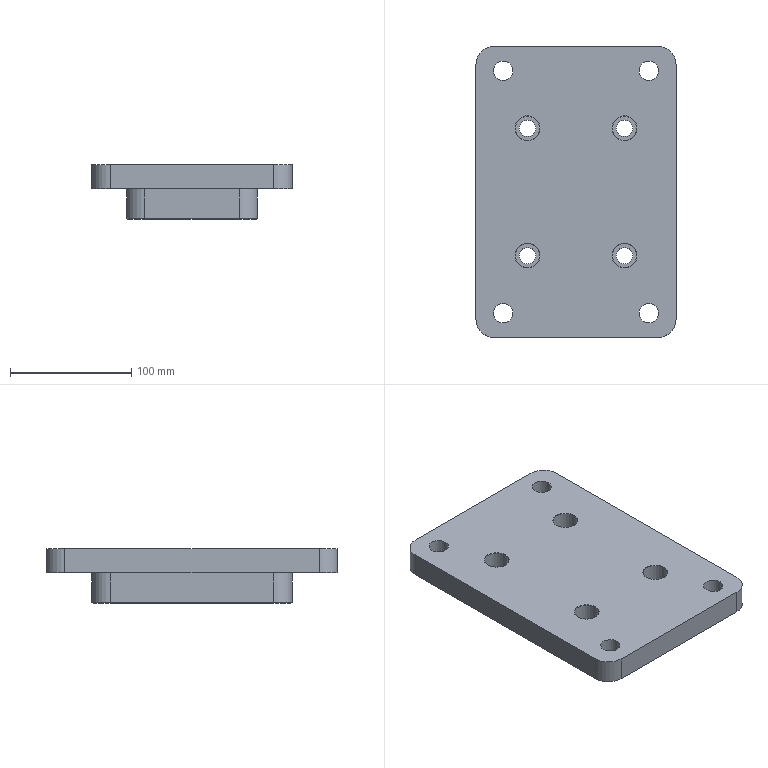Part | 1 solid | 47 faces | box 165 x 240 x 45 mm | volume 1174378 mm3 | cylinder 20 | plane 19 | cone 8 | commonest cylinder face diameters 30 x8 13.5 x4 16 x4 20 x4
STEP:
#1=CARTESIAN_POINT('',(54.,67.5,-20.));
#2=VERTEX_POINT('',#1);
#3=CARTESIAN_POINT('',(54.,67.5,-44.));
#4=VERTEX_POINT('',#3);
#5=CARTESIAN_POINT('',(54.,67.5,-20.));
#6=DIRECTION('',(0.,0.,-1.));
#7=VECTOR('',#6,1000.);
#8=LINE('',#5,#7);
#9=EDGE_CURVE('',#2,#4,#8,.T.);
#10=ORIENTED_EDGE('',*,*,#9,.T.);
#11=CARTESIAN_POINT('',(39.,82.5,-44.));
#12=VERTEX_POINT('',#11);
#13=CARTESIAN_POINT('',(39.,67.5,-44.));
#14=DIRECTION('',(0.,0.,-1.));
#15=DIRECTION('',(-1.,0.,0.));
#16=AXIS2_PLACEMENT_3D('',#13,#14,#15);
#17=CIRCLE('',#16,15.);
#18=EDGE_CURVE('',#4,#12,#17,.F.);
#19=ORIENTED_EDGE('',*,*,#18,.T.);
#20=CARTESIAN_POINT('',(39.,82.5,-20.));
#21=VERTEX_POINT('',#20);
#22=CARTESIAN_POINT('',(39.,82.5,-20.));
#23=DIRECTION('',(0.,0.,-1.));
#24=VECTOR('',#23,1000.);
#25=LINE('',#22,#24);
#26=EDGE_CURVE('',#21,#12,#25,.T.);
#27=ORIENTED_EDGE('',*,*,#26,.F.);
#28=CARTESIAN_POINT('',(39.,67.5,-20.));
#29=DIRECTION('',(0.,0.,1.));
#30=DIRECTION('',(-1.,0.,0.));
#31=AXIS2_PLACEMENT_3D('',#28,#29,#30);
#32=CIRCLE('',#31,15.);
#33=EDGE_CURVE('',#2,#21,#32,.T.);
#34=ORIENTED_EDGE('',*,*,#33,.F.);
#35=EDGE_LOOP('',(#10,#19,#27,#34));
#36=FACE_BOUND('',#35,.T.);
#37=CARTESIAN_POINT('',(39.,67.5,-20.));
#38=DIRECTION('',(0.,0.,-1.));
#39=DIRECTION('',(-1.,0.,0.));
#40=AXIS2_PLACEMENT_3D('',#37,#38,#39);
#41=CYLINDRICAL_SURFACE('',#40,15.);
#42=ADVANCED_FACE('',(#36),#41,.T.);
#43=ORIENTED_EDGE('',*,*,#26,.T.);
#44=CARTESIAN_POINT('',(-39.,82.5,-44.));
#45=VERTEX_POINT('',#44);
#46=CARTESIAN_POINT('',(-39.,82.5,-44.));
#47=DIRECTION('',(-1.,0.,0.));
#48=VECTOR('',#47,1000.);
#49=LINE('',#46,#48);
#50=EDGE_CURVE('',#12,#45,#49,.T.);
#51=ORIENTED_EDGE('',*,*,#50,.T.);
#52=CARTESIAN_POINT('',(-39.,82.5,-20.));
#53=VERTEX_POINT('',#52);
#54=CARTESIAN_POINT('',(-39.,82.5,-20.));
#55=DIRECTION('',(0.,0.,-1.));
#56=VECTOR('',#55,1000.);
#57=LINE('',#54,#56);
#58=EDGE_CURVE('',#53,#45,#57,.T.);
#59=ORIENTED_EDGE('',*,*,#58,.F.);
#60=CARTESIAN_POINT('',(-39.,82.5,-20.));
#61=DIRECTION('',(-1.,0.,0.));
#62=VECTOR('',#61,1000.);
#63=LINE('',#60,#62);
#64=EDGE_CURVE('',#21,#53,#63,.T.);
#65=ORIENTED_EDGE('',*,*,#64,.F.);
#66=EDGE_LOOP('',(#43,#51,#59,#65));
#67=FACE_BOUND('',#66,.T.);
#68=CARTESIAN_POINT('',(-39.,82.5,-20.));
#69=DIRECTION('',(0.,-1.,0.));
#70=DIRECTION('',(0.,0.,-1.));
#71=AXIS2_PLACEMENT_3D('',#68,#69,#70);
#72=PLANE('',#71);
#73=ADVANCED_FACE('',(#67),#72,.F.);
#74=ORIENTED_EDGE('',*,*,#58,.T.);
#75=CARTESIAN_POINT('',(-54.,67.5,-44.));
#76=VERTEX_POINT('',#75);
#77=CARTESIAN_POINT('',(-39.,67.5,-44.));
#78=DIRECTION('',(0.,0.,-1.));
#79=DIRECTION('',(-1.,0.,0.));
#80=AXIS2_PLACEMENT_3D('',#77,#78,#79);
#81=CIRCLE('',#80,15.);
#82=EDGE_CURVE('',#45,#76,#81,.F.);
#83=ORIENTED_EDGE('',*,*,#82,.T.);
#84=CARTESIAN_POINT('',(-54.,67.5,-20.));
#85=VERTEX_POINT('',#84);
#86=CARTESIAN_POINT('',(-54.,67.5,-20.));
#87=DIRECTION('',(0.,0.,-1.));
#88=VECTOR('',#87,1000.);
#89=LINE('',#86,#88);
#90=EDGE_CURVE('',#85,#76,#89,.T.);
#91=ORIENTED_EDGE('',*,*,#90,.F.);
#92=CARTESIAN_POINT('',(-39.,67.5,-20.));
#93=DIRECTION('',(0.,0.,1.));
#94=DIRECTION('',(1.,0.,0.));
#95=AXIS2_PLACEMENT_3D('',#92,#93,#94);
#96=CIRCLE('',#95,15.);
#97=EDGE_CURVE('',#53,#85,#96,.T.);
#98=ORIENTED_EDGE('',*,*,#97,.F.);
#99=EDGE_LOOP('',(#74,#83,#91,#98));
#100=FACE_BOUND('',#99,.T.);
#101=CARTESIAN_POINT('',(-39.,67.5,-20.));
#102=DIRECTION('',(0.,0.,-1.));
#103=DIRECTION('',(-1.,0.,0.));
#104=AXIS2_PLACEMENT_3D('',#101,#102,#103);
#105=CYLINDRICAL_SURFACE('',#104,15.);
#106=ADVANCED_FACE('',(#100),#105,.T.);
#107=ORIENTED_EDGE('',*,*,#90,.T.);
#108=CARTESIAN_POINT('',(-54.,-67.5,-44.));
#109=VERTEX_POINT('',#108);
#110=CARTESIAN_POINT('',(-54.,-67.5,-44.));
#111=DIRECTION('',(0.,-1.,0.));
#112=VECTOR('',#111,1000.);
#113=LINE('',#110,#112);
#114=EDGE_CURVE('',#76,#109,#113,.T.);
#115=ORIENTED_EDGE('',*,*,#114,.T.);
#116=CARTESIAN_POINT('',(-54.,-67.5,-20.));
#117=VERTEX_POINT('',#116);
#118=CARTESIAN_POINT('',(-54.,-67.5,-20.));
#119=DIRECTION('',(0.,0.,-1.));
#120=VECTOR('',#119,1000.);
#121=LINE('',#118,#120);
#122=EDGE_CURVE('',#117,#109,#121,.T.);
#123=ORIENTED_EDGE('',*,*,#122,.F.);
#124=CARTESIAN_POINT('',(-54.,67.5,-20.));
#125=DIRECTION('',(0.,-1.,0.));
#126=VECTOR('',#125,1000.);
#127=LINE('',#124,#126);
#128=EDGE_CURVE('',#85,#117,#127,.T.);
#129=ORIENTED_EDGE('',*,*,#128,.F.);
#130=EDGE_LOOP('',(#107,#115,#123,#129));
#131=FACE_BOUND('',#130,.T.);
#132=CARTESIAN_POINT('',(-54.,67.5,-20.));
#133=DIRECTION('',(1.,0.,0.));
#134=DIRECTION('',(0.,1.,0.));
#135=AXIS2_PLACEMENT_3D('',#132,#133,#134);
#136=PLANE('',#135);
#137=ADVANCED_FACE('',(#131),#136,.F.);
#138=ORIENTED_EDGE('',*,*,#122,.T.);
#139=CARTESIAN_POINT('',(-39.,-82.5,-44.));
#140=VERTEX_POINT('',#139);
#141=CARTESIAN_POINT('',(-39.,-67.5,-44.));
#142=DIRECTION('',(0.,0.,-1.));
#143=DIRECTION('',(-1.,0.,0.));
#144=AXIS2_PLACEMENT_3D('',#141,#142,#143);
#145=CIRCLE('',#144,15.);
#146=EDGE_CURVE('',#109,#140,#145,.F.);
#147=ORIENTED_EDGE('',*,*,#146,.T.);
#148=CARTESIAN_POINT('',(-39.,-82.5,-20.));
#149=VERTEX_POINT('',#148);
#150=CARTESIAN_POINT('',(-39.,-82.5,-20.));
#151=DIRECTION('',(0.,0.,-1.));
#152=VECTOR('',#151,1000.);
#153=LINE('',#150,#152);
#154=EDGE_CURVE('',#149,#140,#153,.T.);
#155=ORIENTED_EDGE('',*,*,#154,.F.);
#156=CARTESIAN_POINT('',(-39.,-67.5,-20.));
#157=DIRECTION('',(0.,0.,1.));
#158=DIRECTION('',(1.,0.,0.));
#159=AXIS2_PLACEMENT_3D('',#156,#157,#158);
#160=CIRCLE('',#159,15.);
#161=EDGE_CURVE('',#117,#149,#160,.T.);
#162=ORIENTED_EDGE('',*,*,#161,.F.);
#163=EDGE_LOOP('',(#138,#147,#155,#162));
#164=FACE_BOUND('',#163,.T.);
#165=CARTESIAN_POINT('',(-39.,-67.5,-20.));
#166=DIRECTION('',(0.,0.,-1.));
#167=DIRECTION('',(-1.,0.,0.));
#168=AXIS2_PLACEMENT_3D('',#165,#166,#167);
#169=CYLINDRICAL_SURFACE('',#168,15.);
#170=ADVANCED_FACE('',(#164),#169,.T.);
#171=ORIENTED_EDGE('',*,*,#154,.T.);
#172=CARTESIAN_POINT('',(39.,-82.5,-44.));
#173=VERTEX_POINT('',#172);
#174=CARTESIAN_POINT('',(39.,-82.5,-44.));
#175=DIRECTION('',(1.,0.,0.));
#176=VECTOR('',#175,1000.);
#177=LINE('',#174,#176);
#178=EDGE_CURVE('',#140,#173,#177,.T.);
#179=ORIENTED_EDGE('',*,*,#178,.T.);
#180=CARTESIAN_POINT('',(39.,-82.5,-20.));
#181=VERTEX_POINT('',#180);
#182=CARTESIAN_POINT('',(39.,-82.5,-20.));
#183=DIRECTION('',(0.,0.,-1.));
#184=VECTOR('',#183,1000.);
#185=LINE('',#182,#184);
#186=EDGE_CURVE('',#181,#173,#185,.T.);
#187=ORIENTED_EDGE('',*,*,#186,.F.);
#188=CARTESIAN_POINT('',(-39.,-82.5,-20.));
#189=DIRECTION('',(1.,0.,0.));
#190=VECTOR('',#189,1000.);
#191=LINE('',#188,#190);
#192=EDGE_CURVE('',#149,#181,#191,.T.);
#193=ORIENTED_EDGE('',*,*,#192,.F.);
#194=EDGE_LOOP('',(#171,#179,#187,#193));
#195=FACE_BOUND('',#194,.T.);
#196=CARTESIAN_POINT('',(-39.,-82.5,-20.));
#197=DIRECTION('',(0.,1.,0.));
#198=DIRECTION('',(0.,0.,1.));
#199=AXIS2_PLACEMENT_3D('',#196,#197,#198);
#200=PLANE('',#199);
#201=ADVANCED_FACE('',(#195),#200,.F.);
#202=ORIENTED_EDGE('',*,*,#186,.T.);
#203=CARTESIAN_POINT('',(54.,-67.5,-44.));
#204=VERTEX_POINT('',#203);
#205=CARTESIAN_POINT('',(39.,-67.5,-44.));
#206=DIRECTION('',(0.,0.,-1.));
#207=DIRECTION('',(-1.,0.,0.));
#208=AXIS2_PLACEMENT_3D('',#205,#206,#207);
#209=CIRCLE('',#208,15.);
#210=EDGE_CURVE('',#173,#204,#209,.F.);
#211=ORIENTED_EDGE('',*,*,#210,.T.);
#212=CARTESIAN_POINT('',(54.,-67.5,-20.));
#213=VERTEX_POINT('',#212);
#214=CARTESIAN_POINT('',(54.,-67.5,-20.));
#215=DIRECTION('',(0.,0.,-1.));
#216=VECTOR('',#215,1000.);
#217=LINE('',#214,#216);
#218=EDGE_CURVE('',#213,#204,#217,.T.);
#219=ORIENTED_EDGE('',*,*,#218,.F.);
#220=CARTESIAN_POINT('',(39.,-67.5,-20.));
#221=DIRECTION('',(0.,0.,1.));
#222=DIRECTION('',(1.,0.,0.));
#223=AXIS2_PLACEMENT_3D('',#220,#221,#222);
#224=CIRCLE('',#223,15.);
#225=EDGE_CURVE('',#181,#213,#224,.T.);
#226=ORIENTED_EDGE('',*,*,#225,.F.);
#227=EDGE_LOOP('',(#202,#211,#219,#226));
#228=FACE_BOUND('',#227,.T.);
#229=CARTESIAN_POINT('',(39.,-67.5,-20.));
#230=DIRECTION('',(0.,0.,-1.));
#231=DIRECTION('',(-1.,0.,0.));
#232=AXIS2_PLACEMENT_3D('',#229,#230,#231);
#233=CYLINDRICAL_SURFACE('',#232,15.);
#234=ADVANCED_FACE('',(#228),#233,.T.);
#235=ORIENTED_EDGE('',*,*,#218,.T.);
#236=CARTESIAN_POINT('',(54.,67.5,-44.));
#237=DIRECTION('',(0.,1.,0.));
#238=VECTOR('',#237,1000.);
#239=LINE('',#236,#238);
#240=EDGE_CURVE('',#204,#4,#239,.T.);
#241=ORIENTED_EDGE('',*,*,#240,.T.);
#242=ORIENTED_EDGE('',*,*,#9,.F.);
#243=CARTESIAN_POINT('',(54.,67.5,-20.));
#244=DIRECTION('',(0.,1.,0.));
#245=VECTOR('',#244,1000.);
#246=LINE('',#243,#245);
#247=EDGE_CURVE('',#213,#2,#246,.T.);
#248=ORIENTED_EDGE('',*,*,#247,.F.);
#249=EDGE_LOOP('',(#235,#241,#242,#248));
#250=FACE_BOUND('',#249,.T.);
#251=CARTESIAN_POINT('',(54.,67.5,-20.));
#252=DIRECTION('',(-1.,0.,0.));
#253=DIRECTION('',(0.,-1.,0.));
#254=AXIS2_PLACEMENT_3D('',#251,#252,#253);
#255=PLANE('',#254);
#256=ADVANCED_FACE('',(#250),#255,.F.);
#257=CARTESIAN_POINT('',(-33.25,52.5,-45.));
#258=VERTEX_POINT('',#257);
#259=CARTESIAN_POINT('',(-40.,52.5,-45.));
#260=DIRECTION('',(0.,0.,1.));
#261=DIRECTION('',(1.,0.,0.));
#262=AXIS2_PLACEMENT_3D('',#259,#260,#261);
#263=CIRCLE('',#262,6.75);
#264=EDGE_CURVE('',#258,#258,#263,.T.);
#265=ORIENTED_EDGE('',*,*,#264,.T.);
#266=EDGE_LOOP('',(#265));
#267=FACE_BOUND('',#266,.T.);
#268=CARTESIAN_POINT('',(46.75,52.5,-45.));
#269=VERTEX_POINT('',#268);
#270=CARTESIAN_POINT('',(40.,52.5,-45.));
#271=DIRECTION('',(0.,0.,1.));
#272=DIRECTION('',(1.,0.,0.));
#273=AXIS2_PLACEMENT_3D('',#270,#271,#272);
#274=CIRCLE('',#273,6.75);
#275=EDGE_CURVE('',#269,#269,#274,.T.);
#276=ORIENTED_EDGE('',*,*,#275,.T.);
#277=EDGE_LOOP('',(#276));
#278=FACE_BOUND('',#277,.T.);
#279=CARTESIAN_POINT('',(-33.25,-52.5,-45.));
#280=VERTEX_POINT('',#279);
#281=CARTESIAN_POINT('',(-40.,-52.5,-45.));
#282=DIRECTION('',(0.,0.,1.));
#283=DIRECTION('',(1.,0.,0.));
#284=AXIS2_PLACEMENT_3D('',#281,#282,#283);
#285=CIRCLE('',#284,6.75);
#286=EDGE_CURVE('',#280,#280,#285,.T.);
#287=ORIENTED_EDGE('',*,*,#286,.T.);
#288=EDGE_LOOP('',(#287));
#289=FACE_BOUND('',#288,.T.);
#290=CARTESIAN_POINT('',(46.75,-52.5,-45.));
#291=VERTEX_POINT('',#290);
#292=CARTESIAN_POINT('',(40.,-52.5,-45.));
#293=DIRECTION('',(0.,0.,1.));
#294=DIRECTION('',(1.,0.,0.));
#295=AXIS2_PLACEMENT_3D('',#292,#293,#294);
#296=CIRCLE('',#295,6.75);
#297=EDGE_CURVE('',#291,#291,#296,.T.);
#298=ORIENTED_EDGE('',*,*,#297,.T.);
#299=EDGE_LOOP('',(#298));
#300=FACE_BOUND('',#299,.T.);
#301=CARTESIAN_POINT('',(39.,81.5,-45.));
#302=VERTEX_POINT('',#301);
#303=CARTESIAN_POINT('',(53.,67.5,-45.));
#304=VERTEX_POINT('',#303);
#305=CARTESIAN_POINT('',(39.,67.5,-45.));
#306=DIRECTION('',(0.,0.,-1.));
#307=DIRECTION('',(-1.,0.,0.));
#308=AXIS2_PLACEMENT_3D('',#305,#306,#307);
#309=CIRCLE('',#308,14.);
#310=EDGE_CURVE('',#302,#304,#309,.T.);
#311=ORIENTED_EDGE('',*,*,#310,.T.);
#312=CARTESIAN_POINT('',(53.,-67.5,-45.));
#313=VERTEX_POINT('',#312);
#314=CARTESIAN_POINT('',(53.,-67.5,-45.));
#315=DIRECTION('',(0.,-1.,0.));
#316=VECTOR('',#315,1000.);
#317=LINE('',#314,#316);
#318=EDGE_CURVE('',#304,#313,#317,.T.);
#319=ORIENTED_EDGE('',*,*,#318,.T.);
#320=CARTESIAN_POINT('',(39.,-81.5,-45.));
#321=VERTEX_POINT('',#320);
#322=CARTESIAN_POINT('',(39.,-67.5,-45.));
#323=DIRECTION('',(0.,0.,-1.));
#324=DIRECTION('',(-1.,0.,0.));
#325=AXIS2_PLACEMENT_3D('',#322,#323,#324);
#326=CIRCLE('',#325,14.);
#327=EDGE_CURVE('',#313,#321,#326,.T.);
#328=ORIENTED_EDGE('',*,*,#327,.T.);
#329=CARTESIAN_POINT('',(-39.,-81.5,-45.));
#330=VERTEX_POINT('',#329);
#331=CARTESIAN_POINT('',(-39.,-81.5,-45.));
#332=DIRECTION('',(-1.,0.,0.));
#333=VECTOR('',#332,1000.);
#334=LINE('',#331,#333);
#335=EDGE_CURVE('',#321,#330,#334,.T.);
#336=ORIENTED_EDGE('',*,*,#335,.T.);
#337=CARTESIAN_POINT('',(-53.,-67.5,-45.));
#338=VERTEX_POINT('',#337);
#339=CARTESIAN_POINT('',(-39.,-67.5,-45.));
#340=DIRECTION('',(0.,0.,-1.));
#341=DIRECTION('',(-1.,0.,0.));
#342=AXIS2_PLACEMENT_3D('',#339,#340,#341);
#343=CIRCLE('',#342,14.);
#344=EDGE_CURVE('',#330,#338,#343,.T.);
#345=ORIENTED_EDGE('',*,*,#344,.T.);
#346=CARTESIAN_POINT('',(-53.,67.5,-45.));
#347=VERTEX_POINT('',#346);
#348=CARTESIAN_POINT('',(-53.,67.5,-45.));
#349=DIRECTION('',(0.,1.,0.));
#350=VECTOR('',#349,1000.);
#351=LINE('',#348,#350);
#352=EDGE_CURVE('',#338,#347,#351,.T.);
#353=ORIENTED_EDGE('',*,*,#352,.T.);
#354=CARTESIAN_POINT('',(-39.,81.5,-45.));
#355=VERTEX_POINT('',#354);
#356=CARTESIAN_POINT('',(-39.,67.5,-45.));
#357=DIRECTION('',(0.,0.,-1.));
#358=DIRECTION('',(-1.,0.,0.));
#359=AXIS2_PLACEMENT_3D('',#356,#357,#358);
#360=CIRCLE('',#359,14.);
#361=EDGE_CURVE('',#347,#355,#360,.T.);
#362=ORIENTED_EDGE('',*,*,#361,.T.);
#363=CARTESIAN_POINT('',(39.,81.5,-45.));
#364=DIRECTION('',(1.,0.,0.));
#365=VECTOR('',#364,1000.);
#366=LINE('',#363,#365);
#367=EDGE_CURVE('',#355,#302,#366,.T.);
#368=ORIENTED_EDGE('',*,*,#367,.T.);
#369=EDGE_LOOP('',(#311,#319,#328,#336,#345,#353,#362,#368));
#370=FACE_BOUND('',#369,.T.);
#371=CARTESIAN_POINT('',(39.,67.5,-45.));
#372=DIRECTION('',(0.,0.,-1.));
#373=DIRECTION('',(-1.,0.,0.));
#374=AXIS2_PLACEMENT_3D('',#371,#372,#373);
#375=PLANE('',#374);
#376=ADVANCED_FACE('',(#267,#278,#289,#300,#370),#375,.T.);
#377=CARTESIAN_POINT('',(-82.5,105.,-20.));
#378=VERTEX_POINT('',#377);
#379=CARTESIAN_POINT('',(-82.5,-105.,-20.));
#380=VERTEX_POINT('',#379);
#381=CARTESIAN_POINT('',(-82.5,120.,-20.));
#382=DIRECTION('',(0.,-1.,0.));
#383=VECTOR('',#382,1000.);
#384=LINE('',#381,#383);
#385=EDGE_CURVE('',#378,#380,#384,.T.);
#386=ORIENTED_EDGE('',*,*,#385,.T.);
#387=CARTESIAN_POINT('',(-82.5,-105.,0.));
#388=VERTEX_POINT('',#387);
#389=CARTESIAN_POINT('',(-82.5,-105.,0.));
#390=DIRECTION('',(0.,0.,-1.));
#391=VECTOR('',#390,1000.);
#392=LINE('',#389,#391);
#393=EDGE_CURVE('',#380,#388,#392,.F.);
#394=ORIENTED_EDGE('',*,*,#393,.T.);
#395=CARTESIAN_POINT('',(-82.5,105.,0.));
#396=VERTEX_POINT('',#395);
#397=CARTESIAN_POINT('',(-82.5,120.,0.));
#398=DIRECTION('',(0.,-1.,0.));
#399=VECTOR('',#398,1000.);
#400=LINE('',#397,#399);
#401=EDGE_CURVE('',#396,#388,#400,.T.);
#402=ORIENTED_EDGE('',*,*,#401,.F.);
#403=CARTESIAN_POINT('',(-82.5,105.,0.));
#404=DIRECTION('',(0.,0.,-1.));
#405=VECTOR('',#404,1000.);
#406=LINE('',#403,#405);
#407=EDGE_CURVE('',#396,#378,#406,.T.);
#408=ORIENTED_EDGE('',*,*,#407,.T.);
#409=EDGE_LOOP('',(#386,#394,#402,#408));
#410=FACE_BOUND('',#409,.T.);
#411=CARTESIAN_POINT('',(-82.5,120.,0.));
#412=DIRECTION('',(1.,0.,0.));
#413=DIRECTION('',(0.,1.,0.));
#414=AXIS2_PLACEMENT_3D('',#411,#412,#413);
#415=PLANE('',#414);
#416=ADVANCED_FACE('',(#410),#415,.F.);
#417=CARTESIAN_POINT('',(-67.5,-120.,-20.));
#418=VERTEX_POINT('',#417);
#419=CARTESIAN_POINT('',(67.5,-120.,-20.));
#420=VERTEX_POINT('',#419);
#421=CARTESIAN_POINT('',(82.5,-120.,-20.));
#422=DIRECTION('',(1.,0.,0.));
#423=VECTOR('',#422,1000.);
#424=LINE('',#421,#423);
#425=EDGE_CURVE('',#418,#420,#424,.T.);
#426=ORIENTED_EDGE('',*,*,#425,.T.);
#427=CARTESIAN_POINT('',(67.5,-120.,0.));
#428=VERTEX_POINT('',#427);
#429=CARTESIAN_POINT('',(67.5,-120.,0.));
#430=DIRECTION('',(0.,0.,-1.));
#431=VECTOR('',#430,1000.);
#432=LINE('',#429,#431);
#433=EDGE_CURVE('',#420,#428,#432,.F.);
#434=ORIENTED_EDGE('',*,*,#433,.T.);
#435=CARTESIAN_POINT('',(-67.5,-120.,0.));
#436=VERTEX_POINT('',#435);
#437=CARTESIAN_POINT('',(82.5,-120.,0.));
#438=DIRECTION('',(1.,0.,0.));
#439=VECTOR('',#438,1000.);
#440=LINE('',#437,#439);
#441=EDGE_CURVE('',#436,#428,#440,.T.);
#442=ORIENTED_EDGE('',*,*,#441,.F.);
#443=CARTESIAN_POINT('',(-67.5,-120.,0.));
#444=DIRECTION('',(0.,0.,-1.));
#445=VECTOR('',#444,1000.);
#446=LINE('',#443,#445);
#447=EDGE_CURVE('',#436,#418,#446,.T.);
#448=ORIENTED_EDGE('',*,*,#447,.T.);
#449=EDGE_LOOP('',(#426,#434,#442,#448));
#450=FACE_BOUND('',#449,.T.);
#451=CARTESIAN_POINT('',(82.5,-120.,0.));
#452=DIRECTION('',(0.,1.,0.));
#453=DIRECTION('',(-1.,0.,0.));
#454=AXIS2_PLACEMENT_3D('',#451,#452,#453);
#455=PLANE('',#454);
#456=ADVANCED_FACE('',(#450),#455,.F.);
#457=CARTESIAN_POINT('',(82.5,-105.,0.));
#458=VERTEX_POINT('',#457);
#459=CARTESIAN_POINT('',(82.5,105.,0.));
#460=VERTEX_POINT('',#459);
#461=CARTESIAN_POINT('',(82.5,120.,0.));
#462=DIRECTION('',(0.,1.,0.));
#463=VECTOR('',#462,1000.);
#464=LINE('',#461,#463);
#465=EDGE_CURVE('',#458,#460,#464,.T.);
#466=ORIENTED_EDGE('',*,*,#465,.F.);
#467=CARTESIAN_POINT('',(82.5,-105.,-20.));
#468=VERTEX_POINT('',#467);
#469=CARTESIAN_POINT('',(82.5,-105.,0.));
#470=DIRECTION('',(0.,0.,-1.));
#471=VECTOR('',#470,1000.);
#472=LINE('',#469,#471);
#473=EDGE_CURVE('',#458,#468,#472,.T.);
#474=ORIENTED_EDGE('',*,*,#473,.T.);
#475=CARTESIAN_POINT('',(82.5,105.,-20.));
#476=VERTEX_POINT('',#475);
#477=CARTESIAN_POINT('',(82.5,120.,-20.));
#478=DIRECTION('',(0.,1.,0.));
#479=VECTOR('',#478,1000.);
#480=LINE('',#477,#479);
#481=EDGE_CURVE('',#468,#476,#480,.T.);
#482=ORIENTED_EDGE('',*,*,#481,.T.);
#483=CARTESIAN_POINT('',(82.5,105.,0.));
#484=DIRECTION('',(0.,0.,-1.));
#485=VECTOR('',#484,1000.);
#486=LINE('',#483,#485);
#487=EDGE_CURVE('',#476,#460,#486,.F.);
#488=ORIENTED_EDGE('',*,*,#487,.T.);
#489=EDGE_LOOP('',(#466,#474,#482,#488));
#490=FACE_BOUND('',#489,.T.);
#491=CARTESIAN_POINT('',(82.5,120.,0.));
#492=DIRECTION('',(-1.,0.,0.));
#493=DIRECTION('',(0.,-1.,0.));
#494=AXIS2_PLACEMENT_3D('',#491,#492,#493);
#495=PLANE('',#494);
#496=ADVANCED_FACE('',(#490),#495,.F.);
#497=CARTESIAN_POINT('',(67.5,120.,0.));
#498=VERTEX_POINT('',#497);
#499=CARTESIAN_POINT('',(-67.5,120.,0.));
#500=VERTEX_POINT('',#499);
#501=CARTESIAN_POINT('',(82.5,120.,0.));
#502=DIRECTION('',(-1.,0.,0.));
#503=VECTOR('',#502,1000.);
#504=LINE('',#501,#503);
#505=EDGE_CURVE('',#498,#500,#504,.T.);
#506=ORIENTED_EDGE('',*,*,#505,.F.);
#507=CARTESIAN_POINT('',(67.5,120.,-20.));
#508=VERTEX_POINT('',#507);
#509=CARTESIAN_POINT('',(67.5,120.,0.));
#510=DIRECTION('',(0.,0.,-1.));
#511=VECTOR('',#510,1000.);
#512=LINE('',#509,#511);
#513=EDGE_CURVE('',#498,#508,#512,.T.);
#514=ORIENTED_EDGE('',*,*,#513,.T.);
#515=CARTESIAN_POINT('',(-67.5,120.,-20.));
#516=VERTEX_POINT('',#515);
#517=CARTESIAN_POINT('',(82.5,120.,-20.));
#518=DIRECTION('',(-1.,0.,0.));
#519=VECTOR('',#518,1000.);
#520=LINE('',#517,#519);
#521=EDGE_CURVE('',#508,#516,#520,.T.);
#522=ORIENTED_EDGE('',*,*,#521,.T.);
#523=CARTESIAN_POINT('',(-67.5,120.,0.));
#524=DIRECTION('',(0.,0.,-1.));
#525=VECTOR('',#524,1000.);
#526=LINE('',#523,#525);
#527=EDGE_CURVE('',#516,#500,#526,.F.);
#528=ORIENTED_EDGE('',*,*,#527,.T.);
#529=EDGE_LOOP('',(#506,#514,#522,#528));
#530=FACE_BOUND('',#529,.T.);
#531=CARTESIAN_POINT('',(82.5,120.,0.));
#532=DIRECTION('',(0.,-1.,0.));
#533=DIRECTION('',(1.,0.,0.));
#534=AXIS2_PLACEMENT_3D('',#531,#532,#533);
#535=PLANE('',#534);
#536=ADVANCED_FACE('',(#530),#535,.F.);
#537=CARTESIAN_POINT('',(-29.75,52.5,0.));
#538=VERTEX_POINT('',#537);
#539=CARTESIAN_POINT('',(-40.,52.5,0.));
#540=DIRECTION('',(0.,0.,1.));
#541=DIRECTION('',(1.,0.,0.));
#542=AXIS2_PLACEMENT_3D('',#539,#540,#541);
#543=CIRCLE('',#542,10.25);
#544=EDGE_CURVE('',#538,#538,#543,.T.);
#545=ORIENTED_EDGE('',*,*,#544,.F.);
#546=EDGE_LOOP('',(#545));
#547=FACE_BOUND('',#546,.T.);
#548=CARTESIAN_POINT('',(50.25,52.5,0.));
#549=VERTEX_POINT('',#548);
#550=CARTESIAN_POINT('',(40.,52.5,0.));
#551=DIRECTION('',(0.,0.,1.));
#552=DIRECTION('',(1.,0.,0.));
#553=AXIS2_PLACEMENT_3D('',#550,#551,#552);
#554=CIRCLE('',#553,10.25);
#555=EDGE_CURVE('',#549,#549,#554,.T.);
#556=ORIENTED_EDGE('',*,*,#555,.F.);
#557=EDGE_LOOP('',(#556));
#558=FACE_BOUND('',#557,.T.);
#559=CARTESIAN_POINT('',(-29.75,-52.5,0.));
#560=VERTEX_POINT('',#559);
#561=CARTESIAN_POINT('',(-40.,-52.5,0.));
#562=DIRECTION('',(0.,0.,1.));
#563=DIRECTION('',(1.,0.,0.));
#564=AXIS2_PLACEMENT_3D('',#561,#562,#563);
#565=CIRCLE('',#564,10.25);
#566=EDGE_CURVE('',#560,#560,#565,.T.);
#567=ORIENTED_EDGE('',*,*,#566,.F.);
#568=EDGE_LOOP('',(#567));
#569=FACE_BOUND('',#568,.T.);
#570=CARTESIAN_POINT('',(50.25,-52.5,0.));
#571=VERTEX_POINT('',#570);
#572=CARTESIAN_POINT('',(40.,-52.5,0.));
#573=DIRECTION('',(0.,0.,1.));
#574=DIRECTION('',(1.,0.,0.));
#575=AXIS2_PLACEMENT_3D('',#572,#573,#574);
#576=CIRCLE('',#575,10.25);
#577=EDGE_CURVE('',#571,#571,#576,.T.);
#578=ORIENTED_EDGE('',*,*,#577,.F.);
#579=EDGE_LOOP('',(#578));
#580=FACE_BOUND('',#579,.T.);
#581=CARTESIAN_POINT('',(-52.,100.,0.));
#582=VERTEX_POINT('',#581);
#583=CARTESIAN_POINT('',(-60.,100.,0.));
#584=DIRECTION('',(0.,0.,-1.));
#585=DIRECTION('',(1.,0.,0.));
#586=AXIS2_PLACEMENT_3D('',#583,#584,#585);
#587=CIRCLE('',#586,8.);
#588=EDGE_CURVE('',#582,#582,#587,.T.);
#589=ORIENTED_EDGE('',*,*,#588,.T.);
#590=EDGE_LOOP('',(#589));
#591=FACE_BOUND('',#590,.T.);
#592=CARTESIAN_POINT('',(52.,100.,0.));
#593=VERTEX_POINT('',#592);
#594=CARTESIAN_POINT('',(60.,100.,0.));
#595=DIRECTION('',(0.,0.,-1.));
#596=DIRECTION('',(-1.,0.,0.));
#597=AXIS2_PLACEMENT_3D('',#594,#595,#596);
#598=CIRCLE('',#597,8.);
#599=EDGE_CURVE('',#593,#593,#598,.T.);
#600=ORIENTED_EDGE('',*,*,#599,.T.);
#601=EDGE_LOOP('',(#600));
#602=FACE_BOUND('',#601,.T.);
#603=CARTESIAN_POINT('',(68.,-100.,0.));
#604=VERTEX_POINT('',#603);
#605=CARTESIAN_POINT('',(60.,-100.,0.));
#606=DIRECTION('',(0.,0.,-1.));
#607=DIRECTION('',(1.,0.,0.));
#608=AXIS2_PLACEMENT_3D('',#605,#606,#607);
#609=CIRCLE('',#608,8.);
#610=EDGE_CURVE('',#604,#604,#609,.T.);
#611=ORIENTED_EDGE('',*,*,#610,.T.);
#612=EDGE_LOOP('',(#611));
#613=FACE_BOUND('',#612,.T.);
#614=CARTESIAN_POINT('',(-68.,-100.,0.));
#615=VERTEX_POINT('',#614);
#616=CARTESIAN_POINT('',(-60.,-100.,0.));
#617=DIRECTION('',(0.,0.,-1.));
#618=DIRECTION('',(-1.,0.,0.));
#619=AXIS2_PLACEMENT_3D('',#616,#617,#618);
#620=CIRCLE('',#619,8.);
#621=EDGE_CURVE('',#615,#615,#620,.T.);
#622=ORIENTED_EDGE('',*,*,#621,.T.);
#623=EDGE_LOOP('',(#622));
#624=FACE_BOUND('',#623,.T.);
#625=ORIENTED_EDGE('',*,*,#441,.T.);
#626=CARTESIAN_POINT('',(67.5,-105.,0.));
#627=DIRECTION('',(0.,0.,-1.));
#628=DIRECTION('',(-1.,0.,0.));
#629=AXIS2_PLACEMENT_3D('',#626,#627,#628);
#630=CIRCLE('',#629,15.);
#631=EDGE_CURVE('',#428,#458,#630,.F.);
#632=ORIENTED_EDGE('',*,*,#631,.T.);
#633=ORIENTED_EDGE('',*,*,#465,.T.);
#634=CARTESIAN_POINT('',(67.5,105.,0.));
#635=DIRECTION('',(0.,0.,-1.));
#636=DIRECTION('',(-1.,0.,0.));
#637=AXIS2_PLACEMENT_3D('',#634,#635,#636);
#638=CIRCLE('',#637,15.);
#639=EDGE_CURVE('',#460,#498,#638,.F.);
#640=ORIENTED_EDGE('',*,*,#639,.T.);
#641=ORIENTED_EDGE('',*,*,#505,.T.);
#642=CARTESIAN_POINT('',(-67.5,105.,0.));
#643=DIRECTION('',(0.,0.,-1.));
#644=DIRECTION('',(-1.,0.,0.));
#645=AXIS2_PLACEMENT_3D('',#642,#643,#644);
#646=CIRCLE('',#645,15.);
#647=EDGE_CURVE('',#500,#396,#646,.F.);
#648=ORIENTED_EDGE('',*,*,#647,.T.);
#649=ORIENTED_EDGE('',*,*,#401,.T.);
#650=CARTESIAN_POINT('',(-67.5,-105.,0.));
#651=DIRECTION('',(0.,0.,-1.));
#652=DIRECTION('',(-1.,0.,0.));
#653=AXIS2_PLACEMENT_3D('',#650,#651,#652);
#654=CIRCLE('',#653,15.);
#655=EDGE_CURVE('',#388,#436,#654,.F.);
#656=ORIENTED_EDGE('',*,*,#655,.T.);
#657=EDGE_LOOP('',(#625,#632,#633,#640,#641,#648,#649,#656));
#658=FACE_BOUND('',#657,.T.);
#659=CARTESIAN_POINT('',(0.,0.,0.));
#660=DIRECTION('',(0.,0.,-1.));
#661=DIRECTION('',(-1.,0.,0.));
#662=AXIS2_PLACEMENT_3D('',#659,#660,#661);
#663=PLANE('',#662);
#664=ADVANCED_FACE('',(#547,#558,#569,#580,#591,#602,#613,#624,#658),#663,.F.);
#665=CARTESIAN_POINT('',(-52.,100.,-20.));
#666=VERTEX_POINT('',#665);
#667=CARTESIAN_POINT('',(-60.,100.,-20.));
#668=DIRECTION('',(0.,0.,-1.));
#669=DIRECTION('',(1.,0.,0.));
#670=AXIS2_PLACEMENT_3D('',#667,#668,#669);
#671=CIRCLE('',#670,8.);
#672=EDGE_CURVE('',#666,#666,#671,.T.);
#673=ORIENTED_EDGE('',*,*,#672,.F.);
#674=EDGE_LOOP('',(#673));
#675=FACE_BOUND('',#674,.T.);
#676=CARTESIAN_POINT('',(52.,100.,-20.));
#677=VERTEX_POINT('',#676);
#678=CARTESIAN_POINT('',(60.,100.,-20.));
#679=DIRECTION('',(0.,0.,-1.));
#680=DIRECTION('',(-1.,0.,0.));
#681=AXIS2_PLACEMENT_3D('',#678,#679,#680);
#682=CIRCLE('',#681,8.);
#683=EDGE_CURVE('',#677,#677,#682,.T.);
#684=ORIENTED_EDGE('',*,*,#683,.F.);
#685=EDGE_LOOP('',(#684));
#686=FACE_BOUND('',#685,.T.);
#687=CARTESIAN_POINT('',(68.,-100.,-20.));
#688=VERTEX_POINT('',#687);
#689=CARTESIAN_POINT('',(60.,-100.,-20.));
#690=DIRECTION('',(0.,0.,-1.));
#691=DIRECTION('',(1.,0.,0.));
#692=AXIS2_PLACEMENT_3D('',#689,#690,#691);
#693=CIRCLE('',#692,8.);
#694=EDGE_CURVE('',#688,#688,#693,.T.);
#695=ORIENTED_EDGE('',*,*,#694,.F.);
#696=EDGE_LOOP('',(#695));
#697=FACE_BOUND('',#696,.T.);
#698=CARTESIAN_POINT('',(-68.,-100.,-20.));
#699=VERTEX_POINT('',#698);
#700=CARTESIAN_POINT('',(-60.,-100.,-20.));
#701=DIRECTION('',(0.,0.,-1.));
#702=DIRECTION('',(-1.,0.,0.));
#703=AXIS2_PLACEMENT_3D('',#700,#701,#702);
#704=CIRCLE('',#703,8.);
#705=EDGE_CURVE('',#699,#699,#704,.T.);
#706=ORIENTED_EDGE('',*,*,#705,.F.);
#707=EDGE_LOOP('',(#706));
#708=FACE_BOUND('',#707,.T.);
#709=ORIENTED_EDGE('',*,*,#247,.T.);
#710=ORIENTED_EDGE('',*,*,#33,.T.);
#711=ORIENTED_EDGE('',*,*,#64,.T.);
#712=ORIENTED_EDGE('',*,*,#97,.T.);
#713=ORIENTED_EDGE('',*,*,#128,.T.);
#714=ORIENTED_EDGE('',*,*,#161,.T.);
#715=ORIENTED_EDGE('',*,*,#192,.T.);
#716=ORIENTED_EDGE('',*,*,#225,.T.);
#717=EDGE_LOOP('',(#709,#710,#711,#712,#713,#714,#715,#716));
#718=FACE_BOUND('',#717,.T.);
#719=ORIENTED_EDGE('',*,*,#481,.F.);
#720=CARTESIAN_POINT('',(67.5,-105.,-20.));
#721=DIRECTION('',(0.,0.,-1.));
#722=DIRECTION('',(-1.,0.,0.));
#723=AXIS2_PLACEMENT_3D('',#720,#721,#722);
#724=CIRCLE('',#723,15.);
#725=EDGE_CURVE('',#468,#420,#724,.T.);
#726=ORIENTED_EDGE('',*,*,#725,.T.);
#727=ORIENTED_EDGE('',*,*,#425,.F.);
#728=CARTESIAN_POINT('',(-67.5,-105.,-20.));
#729=DIRECTION('',(0.,0.,-1.));
#730=DIRECTION('',(-1.,0.,0.));
#731=AXIS2_PLACEMENT_3D('',#728,#729,#730);
#732=CIRCLE('',#731,15.);
#733=EDGE_CURVE('',#418,#380,#732,.T.);
#734=ORIENTED_EDGE('',*,*,#733,.T.);
#735=ORIENTED_EDGE('',*,*,#385,.F.);
#736=CARTESIAN_POINT('',(-67.5,105.,-20.));
#737=DIRECTION('',(0.,0.,-1.));
#738=DIRECTION('',(-1.,0.,0.));
#739=AXIS2_PLACEMENT_3D('',#736,#737,#738);
#740=CIRCLE('',#739,15.);
#741=EDGE_CURVE('',#378,#516,#740,.T.);
#742=ORIENTED_EDGE('',*,*,#741,.T.);
#743=ORIENTED_EDGE('',*,*,#521,.F.);
#744=CARTESIAN_POINT('',(67.5,105.,-20.));
#745=DIRECTION('',(0.,0.,-1.));
#746=DIRECTION('',(-1.,0.,0.));
#747=AXIS2_PLACEMENT_3D('',#744,#745,#746);
#748=CIRCLE('',#747,15.);
#749=EDGE_CURVE('',#508,#476,#748,.T.);
#750=ORIENTED_EDGE('',*,*,#749,.T.);
#751=EDGE_LOOP('',(#719,#726,#727,#734,#735,#742,#743,#750));
#752=FACE_BOUND('',#751,.T.);
#753=CARTESIAN_POINT('',(0.,0.,-20.));
#754=DIRECTION('',(0.,0.,-1.));
#755=DIRECTION('',(-1.,0.,0.));
#756=AXIS2_PLACEMENT_3D('',#753,#754,#755);
#757=PLANE('',#756);
#758=ADVANCED_FACE('',(#675,#686,#697,#708,#718,#752),#757,.T.);
#759=ORIENTED_EDGE('',*,*,#631,.F.);
#760=ORIENTED_EDGE('',*,*,#433,.F.);
#761=ORIENTED_EDGE('',*,*,#725,.F.);
#762=ORIENTED_EDGE('',*,*,#473,.F.);
#763=EDGE_LOOP('',(#759,#760,#761,#762));
#764=FACE_BOUND('',#763,.T.);
#765=CARTESIAN_POINT('',(67.5,-105.,0.));
#766=DIRECTION('',(0.,0.,-1.));
#767=DIRECTION('',(-1.,0.,0.));
#768=AXIS2_PLACEMENT_3D('',#765,#766,#767);
#769=CYLINDRICAL_SURFACE('',#768,15.);
#770=ADVANCED_FACE('',(#764),#769,.T.);
#771=ORIENTED_EDGE('',*,*,#655,.F.);
#772=ORIENTED_EDGE('',*,*,#393,.F.);
#773=ORIENTED_EDGE('',*,*,#733,.F.);
#774=ORIENTED_EDGE('',*,*,#447,.F.);
#775=EDGE_LOOP('',(#771,#772,#773,#774));
#776=FACE_BOUND('',#775,.T.);
#777=CARTESIAN_POINT('',(-67.5,-105.,0.));
#778=DIRECTION('',(0.,0.,-1.));
#779=DIRECTION('',(-1.,0.,0.));
#780=AXIS2_PLACEMENT_3D('',#777,#778,#779);
#781=CYLINDRICAL_SURFACE('',#780,15.);
#782=ADVANCED_FACE('',(#776),#781,.T.);
#783=ORIENTED_EDGE('',*,*,#639,.F.);
#784=ORIENTED_EDGE('',*,*,#487,.F.);
#785=ORIENTED_EDGE('',*,*,#749,.F.);
#786=ORIENTED_EDGE('',*,*,#513,.F.);
#787=EDGE_LOOP('',(#783,#784,#785,#786));
#788=FACE_BOUND('',#787,.T.);
#789=CARTESIAN_POINT('',(67.5,105.,0.));
#790=DIRECTION('',(0.,0.,-1.));
#791=DIRECTION('',(-1.,0.,0.));
#792=AXIS2_PLACEMENT_3D('',#789,#790,#791);
#793=CYLINDRICAL_SURFACE('',#792,15.);
#794=ADVANCED_FACE('',(#788),#793,.T.);
#795=ORIENTED_EDGE('',*,*,#647,.F.);
#796=ORIENTED_EDGE('',*,*,#527,.F.);
#797=ORIENTED_EDGE('',*,*,#741,.F.);
#798=ORIENTED_EDGE('',*,*,#407,.F.);
#799=EDGE_LOOP('',(#795,#796,#797,#798));
#800=FACE_BOUND('',#799,.T.);
#801=CARTESIAN_POINT('',(-67.5,105.,0.));
#802=DIRECTION('',(0.,0.,-1.));
#803=DIRECTION('',(-1.,0.,0.));
#804=AXIS2_PLACEMENT_3D('',#801,#802,#803);
#805=CYLINDRICAL_SURFACE('',#804,15.);
#806=ADVANCED_FACE('',(#800),#805,.T.);
#807=ORIENTED_EDGE('',*,*,#621,.F.);
#808=EDGE_LOOP('',(#807));
#809=FACE_BOUND('',#808,.T.);
#810=ORIENTED_EDGE('',*,*,#705,.T.);
#811=EDGE_LOOP('',(#810));
#812=FACE_BOUND('',#811,.T.);
#813=CARTESIAN_POINT('',(-60.,-100.,0.));
#814=DIRECTION('',(0.,0.,-1.));
#815=DIRECTION('',(-1.,0.,0.));
#816=AXIS2_PLACEMENT_3D('',#813,#814,#815);
#817=CYLINDRICAL_SURFACE('',#816,8.);
#818=ADVANCED_FACE('',(#809,#812),#817,.F.);
#819=ORIENTED_EDGE('',*,*,#610,.F.);
#820=EDGE_LOOP('',(#819));
#821=FACE_BOUND('',#820,.T.);
#822=ORIENTED_EDGE('',*,*,#694,.T.);
#823=EDGE_LOOP('',(#822));
#824=FACE_BOUND('',#823,.T.);
#825=CARTESIAN_POINT('',(60.,-100.,0.));
#826=DIRECTION('',(0.,0.,-1.));
#827=DIRECTION('',(-1.,0.,0.));
#828=AXIS2_PLACEMENT_3D('',#825,#826,#827);
#829=CYLINDRICAL_SURFACE('',#828,8.);
#830=ADVANCED_FACE('',(#821,#824),#829,.F.);
#831=ORIENTED_EDGE('',*,*,#599,.F.);
#832=EDGE_LOOP('',(#831));
#833=FACE_BOUND('',#832,.T.);
#834=ORIENTED_EDGE('',*,*,#683,.T.);
#835=EDGE_LOOP('',(#834));
#836=FACE_BOUND('',#835,.T.);
#837=CARTESIAN_POINT('',(60.,100.,0.));
#838=DIRECTION('',(0.,0.,-1.));
#839=DIRECTION('',(-1.,0.,0.));
#840=AXIS2_PLACEMENT_3D('',#837,#838,#839);
#841=CYLINDRICAL_SURFACE('',#840,8.);
#842=ADVANCED_FACE('',(#833,#836),#841,.F.);
#843=ORIENTED_EDGE('',*,*,#588,.F.);
#844=EDGE_LOOP('',(#843));
#845=FACE_BOUND('',#844,.T.);
#846=ORIENTED_EDGE('',*,*,#672,.T.);
#847=EDGE_LOOP('',(#846));
#848=FACE_BOUND('',#847,.T.);
#849=CARTESIAN_POINT('',(-60.,100.,0.));
#850=DIRECTION('',(0.,0.,-1.));
#851=DIRECTION('',(-1.,0.,0.));
#852=AXIS2_PLACEMENT_3D('',#849,#850,#851);
#853=CYLINDRICAL_SURFACE('',#852,8.);
#854=ADVANCED_FACE('',(#845,#848),#853,.F.);
#855=CARTESIAN_POINT('',(-53.,67.5,-45.));
#856=DIRECTION('',(-0.7071,0.,0.7071));
#857=VECTOR('',#856,1000.);
#858=LINE('',#855,#857);
#859=EDGE_CURVE('',#347,#76,#858,.T.);
#860=ORIENTED_EDGE('',*,*,#859,.F.);
#861=ORIENTED_EDGE('',*,*,#352,.F.);
#862=CARTESIAN_POINT('',(-54.,-67.5,-44.));
#863=DIRECTION('',(0.7071,0.,-0.7071));
#864=VECTOR('',#863,1000.);
#865=LINE('',#862,#864);
#866=EDGE_CURVE('',#109,#338,#865,.T.);
#867=ORIENTED_EDGE('',*,*,#866,.F.);
#868=ORIENTED_EDGE('',*,*,#114,.F.);
#869=EDGE_LOOP('',(#860,#861,#867,#868));
#870=FACE_BOUND('',#869,.T.);
#871=CARTESIAN_POINT('',(-54.,67.5,-44.));
#872=DIRECTION('',(-0.7071,0.,-0.7071));
#873=DIRECTION('',(0.,1.,0.));
#874=AXIS2_PLACEMENT_3D('',#871,#872,#873);
#875=PLANE('',#874);
#876=ADVANCED_FACE('',(#870),#875,.T.);
#877=ORIENTED_EDGE('',*,*,#866,.T.);
#878=ORIENTED_EDGE('',*,*,#344,.F.);
#879=CARTESIAN_POINT('',(-39.,-82.5,-44.));
#880=DIRECTION('',(0.,0.7071,-0.7071));
#881=VECTOR('',#880,1000.);
#882=LINE('',#879,#881);
#883=EDGE_CURVE('',#140,#330,#882,.T.);
#884=ORIENTED_EDGE('',*,*,#883,.F.);
#885=ORIENTED_EDGE('',*,*,#146,.F.);
#886=EDGE_LOOP('',(#877,#878,#884,#885));
#887=FACE_BOUND('',#886,.T.);
#888=CARTESIAN_POINT('',(-39.,-67.5,-44.));
#889=DIRECTION('',(0.,0.,1.));
#890=DIRECTION('',(1.,0.,0.));
#891=AXIS2_PLACEMENT_3D('',#888,#889,#890);
#892=CONICAL_SURFACE('',#891,15.,0.7854);
#893=ADVANCED_FACE('',(#887),#892,.T.);
#894=ORIENTED_EDGE('',*,*,#859,.T.);
#895=ORIENTED_EDGE('',*,*,#82,.F.);
#896=CARTESIAN_POINT('',(-39.,81.5,-45.));
#897=DIRECTION('',(0.,0.7071,0.7071));
#898=VECTOR('',#897,1000.);
#899=LINE('',#896,#898);
#900=EDGE_CURVE('',#355,#45,#899,.T.);
#901=ORIENTED_EDGE('',*,*,#900,.F.);
#902=ORIENTED_EDGE('',*,*,#361,.F.);
#903=EDGE_LOOP('',(#894,#895,#901,#902));
#904=FACE_BOUND('',#903,.T.);
#905=CARTESIAN_POINT('',(-39.,67.5,-44.));
#906=DIRECTION('',(0.,0.,1.));
#907=DIRECTION('',(1.,0.,0.));
#908=AXIS2_PLACEMENT_3D('',#905,#906,#907);
#909=CONICAL_SURFACE('',#908,15.,0.7854);
#910=ADVANCED_FACE('',(#904),#909,.T.);
#911=ORIENTED_EDGE('',*,*,#883,.T.);
#912=ORIENTED_EDGE('',*,*,#335,.F.);
#913=CARTESIAN_POINT('',(39.,-82.5,-44.));
#914=DIRECTION('',(0.,0.7071,-0.7071));
#915=VECTOR('',#914,1000.);
#916=LINE('',#913,#915);
#917=EDGE_CURVE('',#173,#321,#916,.T.);
#918=ORIENTED_EDGE('',*,*,#917,.F.);
#919=ORIENTED_EDGE('',*,*,#178,.F.);
#920=EDGE_LOOP('',(#911,#912,#918,#919));
#921=FACE_BOUND('',#920,.T.);
#922=CARTESIAN_POINT('',(-39.,-82.5,-44.));
#923=DIRECTION('',(0.,-0.7071,-0.7071));
#924=DIRECTION('',(-1.,0.,0.));
#925=AXIS2_PLACEMENT_3D('',#922,#923,#924);
#926=PLANE('',#925);
#927=ADVANCED_FACE('',(#921),#926,.T.);
#928=ORIENTED_EDGE('',*,*,#900,.T.);
#929=ORIENTED_EDGE('',*,*,#50,.F.);
#930=CARTESIAN_POINT('',(39.,81.5,-45.));
#931=DIRECTION('',(0.,0.7071,0.7071));
#932=VECTOR('',#931,1000.);
#933=LINE('',#930,#932);
#934=EDGE_CURVE('',#302,#12,#933,.T.);
#935=ORIENTED_EDGE('',*,*,#934,.F.);
#936=ORIENTED_EDGE('',*,*,#367,.F.);
#937=EDGE_LOOP('',(#928,#929,#935,#936));
#938=FACE_BOUND('',#937,.T.);
#939=CARTESIAN_POINT('',(-39.,82.5,-44.));
#940=DIRECTION('',(0.,0.7071,-0.7071));
#941=DIRECTION('',(1.,0.,0.));
#942=AXIS2_PLACEMENT_3D('',#939,#940,#941);
#943=PLANE('',#942);
#944=ADVANCED_FACE('',(#938),#943,.T.);
#945=ORIENTED_EDGE('',*,*,#917,.T.);
#946=ORIENTED_EDGE('',*,*,#327,.F.);
#947=CARTESIAN_POINT('',(54.,-67.5,-44.));
#948=DIRECTION('',(-0.7071,0.,-0.7071));
#949=VECTOR('',#948,1000.);
#950=LINE('',#947,#949);
#951=EDGE_CURVE('',#204,#313,#950,.T.);
#952=ORIENTED_EDGE('',*,*,#951,.F.);
#953=ORIENTED_EDGE('',*,*,#210,.F.);
#954=EDGE_LOOP('',(#945,#946,#952,#953));
#955=FACE_BOUND('',#954,.T.);
#956=CARTESIAN_POINT('',(39.,-67.5,-44.));
#957=DIRECTION('',(0.,0.,1.));
#958=DIRECTION('',(1.,0.,0.));
#959=AXIS2_PLACEMENT_3D('',#956,#957,#958);
#960=CONICAL_SURFACE('',#959,15.,0.7854);
#961=ADVANCED_FACE('',(#955),#960,.T.);
#962=ORIENTED_EDGE('',*,*,#934,.T.);
#963=ORIENTED_EDGE('',*,*,#18,.F.);
#964=CARTESIAN_POINT('',(53.,67.5,-45.));
#965=DIRECTION('',(0.7071,0.,0.7071));
#966=VECTOR('',#965,1000.);
#967=LINE('',#964,#966);
#968=EDGE_CURVE('',#304,#4,#967,.T.);
#969=ORIENTED_EDGE('',*,*,#968,.F.);
#970=ORIENTED_EDGE('',*,*,#310,.F.);
#971=EDGE_LOOP('',(#962,#963,#969,#970));
#972=FACE_BOUND('',#971,.T.);
#973=CARTESIAN_POINT('',(39.,67.5,-44.));
#974=DIRECTION('',(0.,0.,1.));
#975=DIRECTION('',(1.,0.,0.));
#976=AXIS2_PLACEMENT_3D('',#973,#974,#975);
#977=CONICAL_SURFACE('',#976,15.,0.7854);
#978=ADVANCED_FACE('',(#972),#977,.T.);
#979=ORIENTED_EDGE('',*,*,#951,.T.);
#980=ORIENTED_EDGE('',*,*,#318,.F.);
#981=ORIENTED_EDGE('',*,*,#968,.T.);
#982=ORIENTED_EDGE('',*,*,#240,.F.);
#983=EDGE_LOOP('',(#979,#980,#981,#982));
#984=FACE_BOUND('',#983,.T.);
#985=CARTESIAN_POINT('',(54.,67.5,-44.));
#986=DIRECTION('',(0.7071,0.,-0.7071));
#987=DIRECTION('',(0.,-1.,0.));
#988=AXIS2_PLACEMENT_3D('',#985,#986,#987);
#989=PLANE('',#988);
#990=ADVANCED_FACE('',(#984),#989,.T.);
#991=ORIENTED_EDGE('',*,*,#297,.F.);
#992=EDGE_LOOP('',(#991));
#993=FACE_BOUND('',#992,.T.);
#994=CARTESIAN_POINT('',(46.75,-52.5,-18.));
#995=VERTEX_POINT('',#994);
#996=CARTESIAN_POINT('',(40.,-52.5,-18.));
#997=DIRECTION('',(0.,0.,1.));
#998=DIRECTION('',(1.,0.,0.));
#999=AXIS2_PLACEMENT_3D('',#996,#997,#998);
#1000=CIRCLE('',#999,6.75);
#1001=EDGE_CURVE('',#995,#995,#1000,.T.);
#1002=ORIENTED_EDGE('',*,*,#1001,.T.);
#1003=EDGE_LOOP('',(#1002));
#1004=FACE_BOUND('',#1003,.T.);
#1005=CARTESIAN_POINT('',(40.,-52.5,0.));
#1006=DIRECTION('',(0.,0.,1.));
#1007=DIRECTION('',(1.,0.,0.));
#1008=AXIS2_PLACEMENT_3D('',#1005,#1006,#1007);
#1009=CYLINDRICAL_SURFACE('',#1008,6.75);
#1010=ADVANCED_FACE('',(#993,#1004),#1009,.F.);
#1011=ORIENTED_EDGE('',*,*,#1001,.F.);
#1012=EDGE_LOOP('',(#1011));
#1013=FACE_BOUND('',#1012,.T.);
#1014=CARTESIAN_POINT('',(50.,-52.5,-18.));
#1015=VERTEX_POINT('',#1014);
#1016=CARTESIAN_POINT('',(40.,-52.5,-18.));
#1017=DIRECTION('',(0.,0.,1.));
#1018=DIRECTION('',(1.,0.,0.));
#1019=AXIS2_PLACEMENT_3D('',#1016,#1017,#1018);
#1020=CIRCLE('',#1019,10.);
#1021=EDGE_CURVE('',#1015,#1015,#1020,.T.);
#1022=ORIENTED_EDGE('',*,*,#1021,.T.);
#1023=EDGE_LOOP('',(#1022));
#1024=FACE_BOUND('',#1023,.T.);
#1025=CARTESIAN_POINT('',(50.,-52.5,-18.));
#1026=DIRECTION('',(0.,0.,-1.));
#1027=DIRECTION('',(-1.,0.,0.));
#1028=AXIS2_PLACEMENT_3D('',#1025,#1026,#1027);
#1029=PLANE('',#1028);
#1030=ADVANCED_FACE('',(#1013,#1024),#1029,.F.);
#1031=ORIENTED_EDGE('',*,*,#1021,.F.);
#1032=EDGE_LOOP('',(#1031));
#1033=FACE_BOUND('',#1032,.T.);
#1034=CARTESIAN_POINT('',(50.,-52.5,-0.25));
#1035=VERTEX_POINT('',#1034);
#1036=CARTESIAN_POINT('',(40.,-52.5,-0.25));
#1037=DIRECTION('',(0.,0.,1.));
#1038=DIRECTION('',(1.,0.,0.));
#1039=AXIS2_PLACEMENT_3D('',#1036,#1037,#1038);
#1040=CIRCLE('',#1039,10.);
#1041=EDGE_CURVE('',#1035,#1035,#1040,.T.);
#1042=ORIENTED_EDGE('',*,*,#1041,.T.);
#1043=EDGE_LOOP('',(#1042));
#1044=FACE_BOUND('',#1043,.T.);
#1045=CARTESIAN_POINT('',(40.,-52.5,0.));
#1046=DIRECTION('',(0.,0.,1.));
#1047=DIRECTION('',(1.,0.,0.));
#1048=AXIS2_PLACEMENT_3D('',#1045,#1046,#1047);
#1049=CYLINDRICAL_SURFACE('',#1048,10.);
#1050=ADVANCED_FACE('',(#1033,#1044),#1049,.F.);
#1051=ORIENTED_EDGE('',*,*,#1041,.F.);
#1052=EDGE_LOOP('',(#1051));
#1053=FACE_BOUND('',#1052,.T.);
#1054=ORIENTED_EDGE('',*,*,#577,.T.);
#1055=EDGE_LOOP('',(#1054));
#1056=FACE_BOUND('',#1055,.T.);
#1057=CARTESIAN_POINT('',(40.,-52.5,0.));
#1058=DIRECTION('',(0.,0.,1.));
#1059=DIRECTION('',(1.,0.,0.));
#1060=AXIS2_PLACEMENT_3D('',#1057,#1058,#1059);
#1061=CONICAL_SURFACE('',#1060,10.25,0.7854);
#1062=ADVANCED_FACE('',(#1053,#1056),#1061,.F.);
#1063=ORIENTED_EDGE('',*,*,#286,.F.);
#1064=EDGE_LOOP('',(#1063));
#1065=FACE_BOUND('',#1064,.T.);
#1066=CARTESIAN_POINT('',(-33.25,-52.5,-18.));
#1067=VERTEX_POINT('',#1066);
#1068=CARTESIAN_POINT('',(-40.,-52.5,-18.));
#1069=DIRECTION('',(0.,0.,1.));
#1070=DIRECTION('',(1.,0.,0.));
#1071=AXIS2_PLACEMENT_3D('',#1068,#1069,#1070);
#1072=CIRCLE('',#1071,6.75);
#1073=EDGE_CURVE('',#1067,#1067,#1072,.T.);
#1074=ORIENTED_EDGE('',*,*,#1073,.T.);
#1075=EDGE_LOOP('',(#1074));
#1076=FACE_BOUND('',#1075,.T.);
#1077=CARTESIAN_POINT('',(-40.,-52.5,0.));
#1078=DIRECTION('',(0.,0.,1.));
#1079=DIRECTION('',(1.,0.,0.));
#1080=AXIS2_PLACEMENT_3D('',#1077,#1078,#1079);
#1081=CYLINDRICAL_SURFACE('',#1080,6.75);
#1082=ADVANCED_FACE('',(#1065,#1076),#1081,.F.);
#1083=ORIENTED_EDGE('',*,*,#1073,.F.);
#1084=EDGE_LOOP('',(#1083));
#1085=FACE_BOUND('',#1084,.T.);
#1086=CARTESIAN_POINT('',(-30.,-52.5,-18.));
#1087=VERTEX_POINT('',#1086);
#1088=CARTESIAN_POINT('',(-40.,-52.5,-18.));
#1089=DIRECTION('',(0.,0.,1.));
#1090=DIRECTION('',(1.,0.,0.));
#1091=AXIS2_PLACEMENT_3D('',#1088,#1089,#1090);
#1092=CIRCLE('',#1091,10.);
#1093=EDGE_CURVE('',#1087,#1087,#1092,.T.);
#1094=ORIENTED_EDGE('',*,*,#1093,.T.);
#1095=EDGE_LOOP('',(#1094));
#1096=FACE_BOUND('',#1095,.T.);
#1097=CARTESIAN_POINT('',(-30.,-52.5,-18.));
#1098=DIRECTION('',(0.,0.,-1.));
#1099=DIRECTION('',(-1.,0.,0.));
#1100=AXIS2_PLACEMENT_3D('',#1097,#1098,#1099);
#1101=PLANE('',#1100);
#1102=ADVANCED_FACE('',(#1085,#1096),#1101,.F.);
#1103=ORIENTED_EDGE('',*,*,#1093,.F.);
#1104=EDGE_LOOP('',(#1103));
#1105=FACE_BOUND('',#1104,.T.);
#1106=CARTESIAN_POINT('',(-30.,-52.5,-0.25));
#1107=VERTEX_POINT('',#1106);
#1108=CARTESIAN_POINT('',(-40.,-52.5,-0.25));
#1109=DIRECTION('',(0.,0.,1.));
#1110=DIRECTION('',(1.,0.,0.));
#1111=AXIS2_PLACEMENT_3D('',#1108,#1109,#1110);
#1112=CIRCLE('',#1111,10.);
#1113=EDGE_CURVE('',#1107,#1107,#1112,.T.);
#1114=ORIENTED_EDGE('',*,*,#1113,.T.);
#1115=EDGE_LOOP('',(#1114));
#1116=FACE_BOUND('',#1115,.T.);
#1117=CARTESIAN_POINT('',(-40.,-52.5,0.));
#1118=DIRECTION('',(0.,0.,1.));
#1119=DIRECTION('',(1.,0.,0.));
#1120=AXIS2_PLACEMENT_3D('',#1117,#1118,#1119);
#1121=CYLINDRICAL_SURFACE('',#1120,10.);
#1122=ADVANCED_FACE('',(#1105,#1116),#1121,.F.);
#1123=ORIENTED_EDGE('',*,*,#1113,.F.);
#1124=EDGE_LOOP('',(#1123));
#1125=FACE_BOUND('',#1124,.T.);
#1126=ORIENTED_EDGE('',*,*,#566,.T.);
#1127=EDGE_LOOP('',(#1126));
#1128=FACE_BOUND('',#1127,.T.);
#1129=CARTESIAN_POINT('',(-40.,-52.5,0.));
#1130=DIRECTION('',(0.,0.,1.));
#1131=DIRECTION('',(1.,0.,0.));
#1132=AXIS2_PLACEMENT_3D('',#1129,#1130,#1131);
#1133=CONICAL_SURFACE('',#1132,10.25,0.7854);
#1134=ADVANCED_FACE('',(#1125,#1128),#1133,.F.);
#1135=ORIENTED_EDGE('',*,*,#275,.F.);
#1136=EDGE_LOOP('',(#1135));
#1137=FACE_BOUND('',#1136,.T.);
#1138=CARTESIAN_POINT('',(46.75,52.5,-18.));
#1139=VERTEX_POINT('',#1138);
#1140=CARTESIAN_POINT('',(40.,52.5,-18.));
#1141=DIRECTION('',(0.,0.,1.));
#1142=DIRECTION('',(1.,0.,0.));
#1143=AXIS2_PLACEMENT_3D('',#1140,#1141,#1142);
#1144=CIRCLE('',#1143,6.75);
#1145=EDGE_CURVE('',#1139,#1139,#1144,.T.);
#1146=ORIENTED_EDGE('',*,*,#1145,.T.);
#1147=EDGE_LOOP('',(#1146));
#1148=FACE_BOUND('',#1147,.T.);
#1149=CARTESIAN_POINT('',(40.,52.5,0.));
#1150=DIRECTION('',(0.,0.,1.));
#1151=DIRECTION('',(1.,0.,0.));
#1152=AXIS2_PLACEMENT_3D('',#1149,#1150,#1151);
#1153=CYLINDRICAL_SURFACE('',#1152,6.75);
#1154=ADVANCED_FACE('',(#1137,#1148),#1153,.F.);
#1155=ORIENTED_EDGE('',*,*,#1145,.F.);
#1156=EDGE_LOOP('',(#1155));
#1157=FACE_BOUND('',#1156,.T.);
#1158=CARTESIAN_POINT('',(50.,52.5,-18.));
#1159=VERTEX_POINT('',#1158);
#1160=CARTESIAN_POINT('',(40.,52.5,-18.));
#1161=DIRECTION('',(0.,0.,1.));
#1162=DIRECTION('',(1.,0.,0.));
#1163=AXIS2_PLACEMENT_3D('',#1160,#1161,#1162);
#1164=CIRCLE('',#1163,10.);
#1165=EDGE_CURVE('',#1159,#1159,#1164,.T.);
#1166=ORIENTED_EDGE('',*,*,#1165,.T.);
#1167=EDGE_LOOP('',(#1166));
#1168=FACE_BOUND('',#1167,.T.);
#1169=CARTESIAN_POINT('',(50.,52.5,-18.));
#1170=DIRECTION('',(0.,0.,-1.));
#1171=DIRECTION('',(-1.,0.,0.));
#1172=AXIS2_PLACEMENT_3D('',#1169,#1170,#1171);
#1173=PLANE('',#1172);
#1174=ADVANCED_FACE('',(#1157,#1168),#1173,.F.);
#1175=ORIENTED_EDGE('',*,*,#1165,.F.);
#1176=EDGE_LOOP('',(#1175));
#1177=FACE_BOUND('',#1176,.T.);
#1178=CARTESIAN_POINT('',(50.,52.5,-0.25));
#1179=VERTEX_POINT('',#1178);
#1180=CARTESIAN_POINT('',(40.,52.5,-0.25));
#1181=DIRECTION('',(0.,0.,1.));
#1182=DIRECTION('',(1.,0.,0.));
#1183=AXIS2_PLACEMENT_3D('',#1180,#1181,#1182);
#1184=CIRCLE('',#1183,10.);
#1185=EDGE_CURVE('',#1179,#1179,#1184,.T.);
#1186=ORIENTED_EDGE('',*,*,#1185,.T.);
#1187=EDGE_LOOP('',(#1186));
#1188=FACE_BOUND('',#1187,.T.);
#1189=CARTESIAN_POINT('',(40.,52.5,0.));
#1190=DIRECTION('',(0.,0.,1.));
#1191=DIRECTION('',(1.,0.,0.));
#1192=AXIS2_PLACEMENT_3D('',#1189,#1190,#1191);
#1193=CYLINDRICAL_SURFACE('',#1192,10.);
#1194=ADVANCED_FACE('',(#1177,#1188),#1193,.F.);
#1195=ORIENTED_EDGE('',*,*,#1185,.F.);
#1196=EDGE_LOOP('',(#1195));
#1197=FACE_BOUND('',#1196,.T.);
#1198=ORIENTED_EDGE('',*,*,#555,.T.);
#1199=EDGE_LOOP('',(#1198));
#1200=FACE_BOUND('',#1199,.T.);
#1201=CARTESIAN_POINT('',(40.,52.5,0.));
#1202=DIRECTION('',(0.,0.,1.));
#1203=DIRECTION('',(1.,0.,0.));
#1204=AXIS2_PLACEMENT_3D('',#1201,#1202,#1203);
#1205=CONICAL_SURFACE('',#1204,10.25,0.7854);
#1206=ADVANCED_FACE('',(#1197,#1200),#1205,.F.);
#1207=ORIENTED_EDGE('',*,*,#264,.F.);
#1208=EDGE_LOOP('',(#1207));
#1209=FACE_BOUND('',#1208,.T.);
#1210=CARTESIAN_POINT('',(-33.25,52.5,-18.));
#1211=VERTEX_POINT('',#1210);
#1212=CARTESIAN_POINT('',(-40.,52.5,-18.));
#1213=DIRECTION('',(0.,0.,1.));
#1214=DIRECTION('',(1.,0.,0.));
#1215=AXIS2_PLACEMENT_3D('',#1212,#1213,#1214);
#1216=CIRCLE('',#1215,6.75);
#1217=EDGE_CURVE('',#1211,#1211,#1216,.T.);
#1218=ORIENTED_EDGE('',*,*,#1217,.T.);
#1219=EDGE_LOOP('',(#1218));
#1220=FACE_BOUND('',#1219,.T.);
#1221=CARTESIAN_POINT('',(-40.,52.5,0.));
#1222=DIRECTION('',(0.,0.,1.));
#1223=DIRECTION('',(1.,0.,0.));
#1224=AXIS2_PLACEMENT_3D('',#1221,#1222,#1223);
#1225=CYLINDRICAL_SURFACE('',#1224,6.75);
#1226=ADVANCED_FACE('',(#1209,#1220),#1225,.F.);
#1227=ORIENTED_EDGE('',*,*,#1217,.F.);
#1228=EDGE_LOOP('',(#1227));
#1229=FACE_BOUND('',#1228,.T.);
#1230=CARTESIAN_POINT('',(-30.,52.5,-18.));
#1231=VERTEX_POINT('',#1230);
#1232=CARTESIAN_POINT('',(-40.,52.5,-18.));
#1233=DIRECTION('',(0.,0.,1.));
#1234=DIRECTION('',(1.,0.,0.));
#1235=AXIS2_PLACEMENT_3D('',#1232,#1233,#1234);
#1236=CIRCLE('',#1235,10.);
#1237=EDGE_CURVE('',#1231,#1231,#1236,.T.);
#1238=ORIENTED_EDGE('',*,*,#1237,.T.);
#1239=EDGE_LOOP('',(#1238));
#1240=FACE_BOUND('',#1239,.T.);
#1241=CARTESIAN_POINT('',(-30.,52.5,-18.));
#1242=DIRECTION('',(0.,0.,-1.));
#1243=DIRECTION('',(-1.,0.,0.));
#1244=AXIS2_PLACEMENT_3D('',#1241,#1242,#1243);
#1245=PLANE('',#1244);
#1246=ADVANCED_FACE('',(#1229,#1240),#1245,.F.);
#1247=ORIENTED_EDGE('',*,*,#1237,.F.);
#1248=EDGE_LOOP('',(#1247));
#1249=FACE_BOUND('',#1248,.T.);
#1250=CARTESIAN_POINT('',(-30.,52.5,-0.25));
#1251=VERTEX_POINT('',#1250);
#1252=CARTESIAN_POINT('',(-40.,52.5,-0.25));
#1253=DIRECTION('',(0.,0.,1.));
#1254=DIRECTION('',(1.,0.,0.));
#1255=AXIS2_PLACEMENT_3D('',#1252,#1253,#1254);
#1256=CIRCLE('',#1255,10.);
#1257=EDGE_CURVE('',#1251,#1251,#1256,.T.);
#1258=ORIENTED_EDGE('',*,*,#1257,.T.);
#1259=EDGE_LOOP('',(#1258));
#1260=FACE_BOUND('',#1259,.T.);
#1261=CARTESIAN_POINT('',(-40.,52.5,0.));
#1262=DIRECTION('',(0.,0.,1.));
#1263=DIRECTION('',(1.,0.,0.));
#1264=AXIS2_PLACEMENT_3D('',#1261,#1262,#1263);
#1265=CYLINDRICAL_SURFACE('',#1264,10.);
#1266=ADVANCED_FACE('',(#1249,#1260),#1265,.F.);
#1267=ORIENTED_EDGE('',*,*,#1257,.F.);
#1268=EDGE_LOOP('',(#1267));
#1269=FACE_BOUND('',#1268,.T.);
#1270=ORIENTED_EDGE('',*,*,#544,.T.);
#1271=EDGE_LOOP('',(#1270));
#1272=FACE_BOUND('',#1271,.T.);
#1273=CARTESIAN_POINT('',(-40.,52.5,0.));
#1274=DIRECTION('',(0.,0.,1.));
#1275=DIRECTION('',(1.,0.,0.));
#1276=AXIS2_PLACEMENT_3D('',#1273,#1274,#1275);
#1277=CONICAL_SURFACE('',#1276,10.25,0.7854);
#1278=ADVANCED_FACE('',(#1269,#1272),#1277,.F.);
#1279=CLOSED_SHELL('',(#42,#73,#106,#137,#170,#201,#234,#256,#376,#416,#456,#496,#536,#664,#758,#770,#782,#794,#806,#818,#830,#842,#854,#876,#893,#910,#927,#944,#961,#978,#990,#1010,#1030,#1050,#1062,#1082,#1102,#1122,#1134,#1154,#1174,#1194,#1206,#1226,#1246,#1266,#1278));
#1280=MANIFOLD_SOLID_BREP('',#1279);
#1281=(LENGTH_UNIT()NAMED_UNIT(*)SI_UNIT(.MILLI.,.METRE.));
#1282=UNCERTAINTY_MEASURE_WITH_UNIT(LENGTH_MEASURE(0.00001),#1281,'','');
#1283=(NAMED_UNIT(*)PLANE_ANGLE_UNIT()SI_UNIT($,.RADIAN.));
#1284=(NAMED_UNIT(*)SI_UNIT($,.STERADIAN.)SOLID_ANGLE_UNIT());
#1285=(GEOMETRIC_REPRESENTATION_CONTEXT(3)GLOBAL_UNCERTAINTY_ASSIGNED_CONTEXT((#1282))GLOBAL_UNIT_ASSIGNED_CONTEXT((#1281,#1283,#1284))REPRESENTATION_CONTEXT('',''));
#1286=ADVANCED_BREP_SHAPE_REPRESENTATION('',(#1280),#1285);